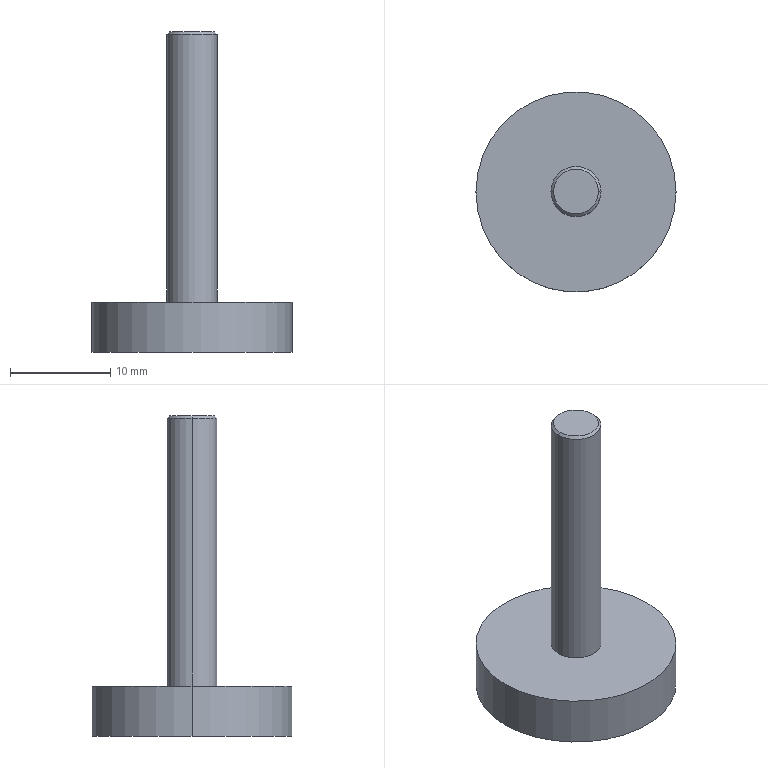Part | SolidWorks | features BaseBody 1 | 1 solid | 9 faces | box 20 x 20 x 32 mm | volume 2100 mm3 | cylinder 4 | plane 3 | cone 2 | commonest cylinder face diameters 5 x2 20 x2
STEP:
#1=CARTESIAN_POINT('',(-2.25,0.,32.));
#2=VERTEX_POINT('',#1);
#3=CARTESIAN_POINT('',(2.25,0.,32.));
#4=VERTEX_POINT('',#3);
#5=CARTESIAN_POINT('',(0.,0.,32.));
#6=DIRECTION('',(0.,0.,-1.));
#7=DIRECTION('',(-1.,0.,0.));
#8=AXIS2_PLACEMENT_3D('',#5,#6,#7);
#9=CIRCLE('',#8,2.25);
#10=EDGE_CURVE('',#2,#4,#9,.T.);
#11=ORIENTED_EDGE('',*,*,#10,.T.);
#12=CARTESIAN_POINT('',(2.5,0.,31.75));
#13=VERTEX_POINT('',#12);
#14=CARTESIAN_POINT('',(2.375,0.,31.875));
#15=DIRECTION('',(0.7071,0.,-0.7071));
#16=VECTOR('',#15,1000.);
#17=LINE('',#14,#16);
#18=EDGE_CURVE('',#4,#13,#17,.T.);
#19=ORIENTED_EDGE('',*,*,#18,.T.);
#20=CARTESIAN_POINT('',(-2.5,0.,31.75));
#21=VERTEX_POINT('',#20);
#22=CARTESIAN_POINT('',(0.,0.,31.75));
#23=DIRECTION('',(0.,0.,1.));
#24=DIRECTION('',(-1.,0.,0.));
#25=AXIS2_PLACEMENT_3D('',#22,#23,#24);
#26=CIRCLE('',#25,2.5);
#27=EDGE_CURVE('',#13,#21,#26,.T.);
#28=ORIENTED_EDGE('',*,*,#27,.T.);
#29=CARTESIAN_POINT('',(-2.375,0.,31.875));
#30=DIRECTION('',(-0.7071,0.,-0.7071));
#31=VECTOR('',#30,1000.);
#32=LINE('',#29,#31);
#33=EDGE_CURVE('',#2,#21,#32,.T.);
#34=ORIENTED_EDGE('',*,*,#33,.F.);
#35=EDGE_LOOP('',(#11,#19,#28,#34));
#36=FACE_OUTER_BOUND('',#35,.T.);
#37=CARTESIAN_POINT('',(0.,0.,31.875));
#38=DIRECTION('',(0.,0.,-1.));
#39=DIRECTION('',(-1.,0.,0.));
#40=AXIS2_PLACEMENT_3D('',#37,#38,#39);
#41=CONICAL_SURFACE('',#40,2.375,0.7854);
#42=ADVANCED_FACE('',(#36),#41,.T.);
#43=ORIENTED_EDGE('',*,*,#27,.F.);
#44=CARTESIAN_POINT('',(2.5,0.,5.));
#45=VERTEX_POINT('',#44);
#46=CARTESIAN_POINT('',(2.5,0.,5.));
#47=DIRECTION('',(0.,0.,-1.));
#48=VECTOR('',#47,1000.);
#49=LINE('',#46,#48);
#50=EDGE_CURVE('',#13,#45,#49,.T.);
#51=ORIENTED_EDGE('',*,*,#50,.T.);
#52=CARTESIAN_POINT('',(-2.5,0.,5.));
#53=VERTEX_POINT('',#52);
#54=CARTESIAN_POINT('',(0.,0.,5.));
#55=DIRECTION('',(0.,0.,-1.));
#56=DIRECTION('',(-1.,0.,0.));
#57=AXIS2_PLACEMENT_3D('',#54,#55,#56);
#58=CIRCLE('',#57,2.5);
#59=EDGE_CURVE('',#53,#45,#58,.T.);
#60=ORIENTED_EDGE('',*,*,#59,.F.);
#61=CARTESIAN_POINT('',(-2.5,0.,5.));
#62=DIRECTION('',(0.,0.,-1.));
#63=VECTOR('',#62,1000.);
#64=LINE('',#61,#63);
#65=EDGE_CURVE('',#21,#53,#64,.T.);
#66=ORIENTED_EDGE('',*,*,#65,.F.);
#67=EDGE_LOOP('',(#43,#51,#60,#66));
#68=FACE_OUTER_BOUND('',#67,.T.);
#69=CARTESIAN_POINT('',(0.,0.,5.));
#70=DIRECTION('',(0.,0.,-1.));
#71=DIRECTION('',(-1.,0.,0.));
#72=AXIS2_PLACEMENT_3D('',#69,#70,#71);
#73=CYLINDRICAL_SURFACE('',#72,2.5);
#74=ADVANCED_FACE('',(#68),#73,.T.);
#75=CARTESIAN_POINT('',(10.,0.,5.));
#76=VERTEX_POINT('',#75);
#77=CARTESIAN_POINT('',(-10.,0.,5.));
#78=VERTEX_POINT('',#77);
#79=CARTESIAN_POINT('',(0.,0.,5.));
#80=DIRECTION('',(0.,0.,1.));
#81=DIRECTION('',(-1.,0.,0.));
#82=AXIS2_PLACEMENT_3D('',#79,#80,#81);
#83=CIRCLE('',#82,10.);
#84=EDGE_CURVE('',#76,#78,#83,.T.);
#85=ORIENTED_EDGE('',*,*,#84,.F.);
#86=CARTESIAN_POINT('',(10.,0.,0.));
#87=VERTEX_POINT('',#86);
#88=CARTESIAN_POINT('',(10.,0.,0.));
#89=DIRECTION('',(0.,0.,-1.));
#90=VECTOR('',#89,1000.);
#91=LINE('',#88,#90);
#92=EDGE_CURVE('',#76,#87,#91,.T.);
#93=ORIENTED_EDGE('',*,*,#92,.T.);
#94=CARTESIAN_POINT('',(-10.,0.,0.));
#95=VERTEX_POINT('',#94);
#96=CARTESIAN_POINT('',(0.,0.,0.));
#97=DIRECTION('',(0.,0.,-1.));
#98=DIRECTION('',(-1.,0.,0.));
#99=AXIS2_PLACEMENT_3D('',#96,#97,#98);
#100=CIRCLE('',#99,10.);
#101=EDGE_CURVE('',#95,#87,#100,.T.);
#102=ORIENTED_EDGE('',*,*,#101,.F.);
#103=CARTESIAN_POINT('',(-10.,0.,0.));
#104=DIRECTION('',(0.,0.,-1.));
#105=VECTOR('',#104,1000.);
#106=LINE('',#103,#105);
#107=EDGE_CURVE('',#78,#95,#106,.T.);
#108=ORIENTED_EDGE('',*,*,#107,.F.);
#109=EDGE_LOOP('',(#85,#93,#102,#108));
#110=FACE_OUTER_BOUND('',#109,.T.);
#111=CARTESIAN_POINT('',(0.,0.,0.));
#112=DIRECTION('',(0.,0.,-1.));
#113=DIRECTION('',(-1.,0.,0.));
#114=AXIS2_PLACEMENT_3D('',#111,#112,#113);
#115=CYLINDRICAL_SURFACE('',#114,10.);
#116=ADVANCED_FACE('',(#110),#115,.T.);
#117=ORIENTED_EDGE('',*,*,#10,.F.);
#118=CARTESIAN_POINT('',(0.,0.,32.));
#119=DIRECTION('',(0.,0.,-1.));
#120=DIRECTION('',(-1.,0.,0.));
#121=AXIS2_PLACEMENT_3D('',#118,#119,#120);
#122=CIRCLE('',#121,2.25);
#123=EDGE_CURVE('',#4,#2,#122,.T.);
#124=ORIENTED_EDGE('',*,*,#123,.F.);
#125=EDGE_LOOP('',(#117,#124));
#126=FACE_OUTER_BOUND('',#125,.T.);
#127=CARTESIAN_POINT('',(0.,0.,32.));
#128=DIRECTION('',(0.,0.,1.));
#129=DIRECTION('',(1.,0.,0.));
#130=AXIS2_PLACEMENT_3D('',#127,#128,#129);
#131=PLANE('',#130);
#132=ADVANCED_FACE('',(#126),#131,.T.);
#133=ORIENTED_EDGE('',*,*,#101,.T.);
#134=CARTESIAN_POINT('',(0.,0.,0.));
#135=DIRECTION('',(0.,0.,-1.));
#136=DIRECTION('',(-1.,0.,0.));
#137=AXIS2_PLACEMENT_3D('',#134,#135,#136);
#138=CIRCLE('',#137,10.);
#139=EDGE_CURVE('',#87,#95,#138,.T.);
#140=ORIENTED_EDGE('',*,*,#139,.T.);
#141=EDGE_LOOP('',(#133,#140));
#142=FACE_OUTER_BOUND('',#141,.T.);
#143=CARTESIAN_POINT('',(0.,0.,0.));
#144=DIRECTION('',(0.,0.,1.));
#145=DIRECTION('',(1.,0.,0.));
#146=AXIS2_PLACEMENT_3D('',#143,#144,#145);
#147=PLANE('',#146);
#148=ADVANCED_FACE('',(#142),#147,.F.);
#149=ORIENTED_EDGE('',*,*,#59,.T.);
#150=CARTESIAN_POINT('',(0.,0.,5.));
#151=DIRECTION('',(0.,0.,-1.));
#152=DIRECTION('',(-1.,0.,0.));
#153=AXIS2_PLACEMENT_3D('',#150,#151,#152);
#154=CIRCLE('',#153,2.5);
#155=EDGE_CURVE('',#45,#53,#154,.T.);
#156=ORIENTED_EDGE('',*,*,#155,.T.);
#157=EDGE_LOOP('',(#149,#156));
#158=FACE_BOUND('',#157,.T.);
#159=CARTESIAN_POINT('',(0.,0.,5.));
#160=DIRECTION('',(0.,0.,1.));
#161=DIRECTION('',(-1.,0.,0.));
#162=AXIS2_PLACEMENT_3D('',#159,#160,#161);
#163=CIRCLE('',#162,10.);
#164=EDGE_CURVE('',#78,#76,#163,.T.);
#165=ORIENTED_EDGE('',*,*,#164,.T.);
#166=ORIENTED_EDGE('',*,*,#84,.T.);
#167=EDGE_LOOP('',(#165,#166));
#168=FACE_OUTER_BOUND('',#167,.T.);
#169=CARTESIAN_POINT('',(0.,0.,5.));
#170=DIRECTION('',(0.,0.,1.));
#171=DIRECTION('',(1.,0.,0.));
#172=AXIS2_PLACEMENT_3D('',#169,#170,#171);
#173=PLANE('',#172);
#174=ADVANCED_FACE('',(#158,#168),#173,.T.);
#175=ORIENTED_EDGE('',*,*,#92,.F.);
#176=ORIENTED_EDGE('',*,*,#164,.F.);
#177=ORIENTED_EDGE('',*,*,#107,.T.);
#178=ORIENTED_EDGE('',*,*,#139,.F.);
#179=EDGE_LOOP('',(#175,#176,#177,#178));
#180=FACE_OUTER_BOUND('',#179,.T.);
#181=CARTESIAN_POINT('',(0.,0.,0.));
#182=DIRECTION('',(0.,0.,-1.));
#183=DIRECTION('',(-1.,0.,0.));
#184=AXIS2_PLACEMENT_3D('',#181,#182,#183);
#185=CYLINDRICAL_SURFACE('',#184,10.);
#186=ADVANCED_FACE('',(#180),#185,.T.);
#187=ORIENTED_EDGE('',*,*,#50,.F.);
#188=CARTESIAN_POINT('',(0.,0.,31.75));
#189=DIRECTION('',(0.,0.,1.));
#190=DIRECTION('',(-1.,0.,0.));
#191=AXIS2_PLACEMENT_3D('',#188,#189,#190);
#192=CIRCLE('',#191,2.5);
#193=EDGE_CURVE('',#21,#13,#192,.T.);
#194=ORIENTED_EDGE('',*,*,#193,.F.);
#195=ORIENTED_EDGE('',*,*,#65,.T.);
#196=ORIENTED_EDGE('',*,*,#155,.F.);
#197=EDGE_LOOP('',(#187,#194,#195,#196));
#198=FACE_OUTER_BOUND('',#197,.T.);
#199=CARTESIAN_POINT('',(0.,0.,5.));
#200=DIRECTION('',(0.,0.,-1.));
#201=DIRECTION('',(-1.,0.,0.));
#202=AXIS2_PLACEMENT_3D('',#199,#200,#201);
#203=CYLINDRICAL_SURFACE('',#202,2.5);
#204=ADVANCED_FACE('',(#198),#203,.T.);
#205=ORIENTED_EDGE('',*,*,#18,.F.);
#206=ORIENTED_EDGE('',*,*,#123,.T.);
#207=ORIENTED_EDGE('',*,*,#33,.T.);
#208=ORIENTED_EDGE('',*,*,#193,.T.);
#209=EDGE_LOOP('',(#205,#206,#207,#208));
#210=FACE_OUTER_BOUND('',#209,.T.);
#211=CARTESIAN_POINT('',(0.,0.,31.875));
#212=DIRECTION('',(0.,0.,-1.));
#213=DIRECTION('',(-1.,0.,0.));
#214=AXIS2_PLACEMENT_3D('',#211,#212,#213);
#215=CONICAL_SURFACE('',#214,2.375,0.7854);
#216=ADVANCED_FACE('',(#210),#215,.T.);
#217=CLOSED_SHELL('',(#42,#74,#116,#132,#148,#174,#186,#204,#216));
#218=MANIFOLD_SOLID_BREP('',#217);
#219=CARTESIAN_POINT('',(0.,0.,0.));
#220=DIRECTION('',(0.,0.,1.));
#221=DIRECTION('',(1.,0.,0.));
#222=AXIS2_PLACEMENT_3D('',#219,#220,#221);
#223=(LENGTH_UNIT()NAMED_UNIT(*)SI_UNIT(.MILLI.,.METRE.));
#224=UNCERTAINTY_MEASURE_WITH_UNIT(LENGTH_MEASURE(0.00001),#223,'','');
#225=(NAMED_UNIT(*)PLANE_ANGLE_UNIT()SI_UNIT($,.RADIAN.));
#226=(NAMED_UNIT(*)SI_UNIT($,.STERADIAN.)SOLID_ANGLE_UNIT());
#227=(GEOMETRIC_REPRESENTATION_CONTEXT(3)GLOBAL_UNCERTAINTY_ASSIGNED_CONTEXT((#224))GLOBAL_UNIT_ASSIGNED_CONTEXT((#223,#225,#226))REPRESENTATION_CONTEXT('',''));
#228=ADVANCED_BREP_SHAPE_REPRESENTATION('',(#218,#222),#227);